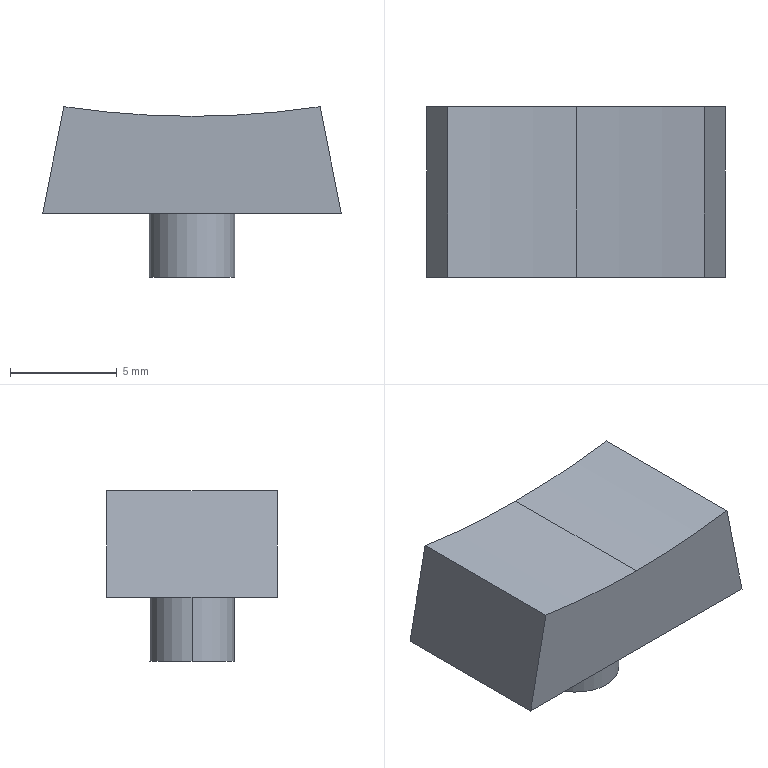Part | SolidWorks | features Extrusion 1, ICE 1 | 1 solid | 13 faces | box 14 x 8 x 8 mm | volume 507.497 mm3 | plane 7 | cylinder 6 | commonest cylinder face diameters 3 x2 4 x2 80 x2
STEP:
#1=CARTESIAN_POINT('',(-1.5,0.,-3.));
#2=VERTEX_POINT('',#1);
#3=CARTESIAN_POINT('',(1.5,0.,-3.));
#4=VERTEX_POINT('',#3);
#5=CARTESIAN_POINT('',(0.,0.,-3.));
#6=DIRECTION('',(0.,0.,1.));
#7=DIRECTION('',(1.,0.,0.));
#8=AXIS2_PLACEMENT_3D('',#5,#6,#7);
#9=CIRCLE('',#8,1.5);
#10=EDGE_CURVE('',#2,#4,#9,.T.);
#11=ORIENTED_EDGE('',*,*,#10,.F.);
#12=CARTESIAN_POINT('',(-1.5,0.,0.));
#13=VERTEX_POINT('',#12);
#14=CARTESIAN_POINT('',(-1.5,0.,-3.));
#15=DIRECTION('',(0.,0.,1.));
#16=VECTOR('',#15,1000.);
#17=LINE('',#14,#16);
#18=EDGE_CURVE('',#2,#13,#17,.T.);
#19=ORIENTED_EDGE('',*,*,#18,.T.);
#20=CARTESIAN_POINT('',(1.5,0.,0.));
#21=VERTEX_POINT('',#20);
#22=CARTESIAN_POINT('',(0.,0.,0.));
#23=DIRECTION('',(0.,0.,1.));
#24=DIRECTION('',(1.,0.,0.));
#25=AXIS2_PLACEMENT_3D('',#22,#23,#24);
#26=CIRCLE('',#25,1.5);
#27=EDGE_CURVE('',#13,#21,#26,.T.);
#28=ORIENTED_EDGE('',*,*,#27,.T.);
#29=CARTESIAN_POINT('',(1.5,0.,-3.));
#30=DIRECTION('',(0.,0.,1.));
#31=VECTOR('',#30,1000.);
#32=LINE('',#29,#31);
#33=EDGE_CURVE('',#4,#21,#32,.T.);
#34=ORIENTED_EDGE('',*,*,#33,.F.);
#35=EDGE_LOOP('',(#11,#19,#28,#34));
#36=FACE_OUTER_BOUND('',#35,.T.);
#37=CARTESIAN_POINT('',(0.,0.,-3.));
#38=DIRECTION('',(0.,0.,1.));
#39=DIRECTION('',(1.,0.,0.));
#40=AXIS2_PLACEMENT_3D('',#37,#38,#39);
#41=CYLINDRICAL_SURFACE('',#40,1.5);
#42=ADVANCED_FACE('',(#36),#41,.F.);
#43=CARTESIAN_POINT('',(2.,0.,-3.));
#44=VERTEX_POINT('',#43);
#45=CARTESIAN_POINT('',(-2.,0.,-3.));
#46=VERTEX_POINT('',#45);
#47=CARTESIAN_POINT('',(0.,0.,-3.));
#48=DIRECTION('',(0.,0.,1.));
#49=DIRECTION('',(1.,0.,0.));
#50=AXIS2_PLACEMENT_3D('',#47,#48,#49);
#51=CIRCLE('',#50,2.);
#52=EDGE_CURVE('',#44,#46,#51,.T.);
#53=ORIENTED_EDGE('',*,*,#52,.T.);
#54=CARTESIAN_POINT('',(-2.,0.,0.));
#55=VERTEX_POINT('',#54);
#56=CARTESIAN_POINT('',(-2.,0.,-3.));
#57=DIRECTION('',(0.,0.,1.));
#58=VECTOR('',#57,1000.);
#59=LINE('',#56,#58);
#60=EDGE_CURVE('',#46,#55,#59,.T.);
#61=ORIENTED_EDGE('',*,*,#60,.T.);
#62=CARTESIAN_POINT('',(2.,0.,0.));
#63=VERTEX_POINT('',#62);
#64=CARTESIAN_POINT('',(0.,0.,0.));
#65=DIRECTION('',(0.,0.,1.));
#66=DIRECTION('',(1.,0.,0.));
#67=AXIS2_PLACEMENT_3D('',#64,#65,#66);
#68=CIRCLE('',#67,2.);
#69=EDGE_CURVE('',#63,#55,#68,.T.);
#70=ORIENTED_EDGE('',*,*,#69,.F.);
#71=CARTESIAN_POINT('',(2.,0.,-3.));
#72=DIRECTION('',(0.,0.,1.));
#73=VECTOR('',#72,1000.);
#74=LINE('',#71,#73);
#75=EDGE_CURVE('',#44,#63,#74,.T.);
#76=ORIENTED_EDGE('',*,*,#75,.F.);
#77=EDGE_LOOP('',(#53,#61,#70,#76));
#78=FACE_OUTER_BOUND('',#77,.T.);
#79=CARTESIAN_POINT('',(0.,0.,-3.));
#80=DIRECTION('',(0.,0.,1.));
#81=DIRECTION('',(1.,0.,0.));
#82=AXIS2_PLACEMENT_3D('',#79,#80,#81);
#83=CYLINDRICAL_SURFACE('',#82,2.);
#84=ADVANCED_FACE('',(#78),#83,.T.);
#85=CARTESIAN_POINT('',(0.,4.,4.547));
#86=VERTEX_POINT('',#85);
#87=CARTESIAN_POINT('',(6.,4.,5.));
#88=VERTEX_POINT('',#87);
#89=CARTESIAN_POINT('',(0.,4.,44.547));
#90=DIRECTION('',(0.,-1.,0.));
#91=DIRECTION('',(0.,0.,-1.));
#92=AXIS2_PLACEMENT_3D('',#89,#90,#91);
#93=CIRCLE('',#92,40.);
#94=EDGE_CURVE('',#86,#88,#93,.T.);
#95=ORIENTED_EDGE('',*,*,#94,.F.);
#96=CARTESIAN_POINT('',(0.,-4.,4.547));
#97=VERTEX_POINT('',#96);
#98=CARTESIAN_POINT('',(0.,4.,4.547));
#99=DIRECTION('',(0.,-1.,0.));
#100=VECTOR('',#99,1000.);
#101=LINE('',#98,#100);
#102=EDGE_CURVE('',#86,#97,#101,.T.);
#103=ORIENTED_EDGE('',*,*,#102,.T.);
#104=CARTESIAN_POINT('',(6.,-4.,5.));
#105=VERTEX_POINT('',#104);
#106=CARTESIAN_POINT('',(0.,-4.,44.547));
#107=DIRECTION('',(0.,-1.,0.));
#108=DIRECTION('',(0.,0.,-1.));
#109=AXIS2_PLACEMENT_3D('',#106,#107,#108);
#110=CIRCLE('',#109,40.);
#111=EDGE_CURVE('',#97,#105,#110,.T.);
#112=ORIENTED_EDGE('',*,*,#111,.T.);
#113=CARTESIAN_POINT('',(6.,4.,5.));
#114=DIRECTION('',(0.,-1.,0.));
#115=VECTOR('',#114,1000.);
#116=LINE('',#113,#115);
#117=EDGE_CURVE('',#88,#105,#116,.T.);
#118=ORIENTED_EDGE('',*,*,#117,.F.);
#119=EDGE_LOOP('',(#95,#103,#112,#118));
#120=FACE_OUTER_BOUND('',#119,.T.);
#121=CARTESIAN_POINT('',(0.,4.,44.547));
#122=DIRECTION('',(0.,-1.,0.));
#123=DIRECTION('',(0.,0.,-1.));
#124=AXIS2_PLACEMENT_3D('',#121,#122,#123);
#125=CYLINDRICAL_SURFACE('',#124,40.);
#126=ADVANCED_FACE('',(#120),#125,.F.);
#127=CARTESIAN_POINT('',(7.,-4.,0.));
#128=VERTEX_POINT('',#127);
#129=CARTESIAN_POINT('',(7.,-4.,0.));
#130=DIRECTION('',(0.1961,0.,-0.9806));
#131=VECTOR('',#130,1000.);
#132=LINE('',#129,#131);
#133=EDGE_CURVE('',#105,#128,#132,.T.);
#134=ORIENTED_EDGE('',*,*,#133,.T.);
#135=CARTESIAN_POINT('',(7.,4.,0.));
#136=VERTEX_POINT('',#135);
#137=CARTESIAN_POINT('',(7.,4.,0.));
#138=DIRECTION('',(0.,-1.,0.));
#139=VECTOR('',#138,1000.);
#140=LINE('',#137,#139);
#141=EDGE_CURVE('',#136,#128,#140,.T.);
#142=ORIENTED_EDGE('',*,*,#141,.F.);
#143=CARTESIAN_POINT('',(7.,4.,0.));
#144=DIRECTION('',(0.1961,0.,-0.9806));
#145=VECTOR('',#144,1000.);
#146=LINE('',#143,#145);
#147=EDGE_CURVE('',#88,#136,#146,.T.);
#148=ORIENTED_EDGE('',*,*,#147,.F.);
#149=ORIENTED_EDGE('',*,*,#117,.T.);
#150=EDGE_LOOP('',(#134,#142,#148,#149));
#151=FACE_OUTER_BOUND('',#150,.T.);
#152=CARTESIAN_POINT('',(7.,4.,0.));
#153=DIRECTION('',(-0.9806,0.,-0.1961));
#154=DIRECTION('',(-0.1961,0.,0.9806));
#155=AXIS2_PLACEMENT_3D('',#152,#153,#154);
#156=PLANE('',#155);
#157=ADVANCED_FACE('',(#151),#156,.F.);
#158=ORIENTED_EDGE('',*,*,#69,.T.);
#159=CARTESIAN_POINT('',(0.,0.,0.));
#160=DIRECTION('',(0.,0.,1.));
#161=DIRECTION('',(1.,0.,0.));
#162=AXIS2_PLACEMENT_3D('',#159,#160,#161);
#163=CIRCLE('',#162,2.);
#164=EDGE_CURVE('',#55,#63,#163,.T.);
#165=ORIENTED_EDGE('',*,*,#164,.T.);
#166=EDGE_LOOP('',(#158,#165));
#167=FACE_BOUND('',#166,.T.);
#168=CARTESIAN_POINT('',(-7.,-4.,0.));
#169=VERTEX_POINT('',#168);
#170=CARTESIAN_POINT('',(7.,-4.,0.));
#171=DIRECTION('',(-1.,0.,0.));
#172=VECTOR('',#171,1000.);
#173=LINE('',#170,#172);
#174=EDGE_CURVE('',#128,#169,#173,.T.);
#175=ORIENTED_EDGE('',*,*,#174,.T.);
#176=CARTESIAN_POINT('',(-7.,4.,0.));
#177=VERTEX_POINT('',#176);
#178=CARTESIAN_POINT('',(-7.,4.,0.));
#179=DIRECTION('',(0.,-1.,0.));
#180=VECTOR('',#179,1000.);
#181=LINE('',#178,#180);
#182=EDGE_CURVE('',#177,#169,#181,.T.);
#183=ORIENTED_EDGE('',*,*,#182,.F.);
#184=CARTESIAN_POINT('',(7.,4.,0.));
#185=DIRECTION('',(-1.,0.,0.));
#186=VECTOR('',#185,1000.);
#187=LINE('',#184,#186);
#188=EDGE_CURVE('',#136,#177,#187,.T.);
#189=ORIENTED_EDGE('',*,*,#188,.F.);
#190=ORIENTED_EDGE('',*,*,#141,.T.);
#191=EDGE_LOOP('',(#175,#183,#189,#190));
#192=FACE_OUTER_BOUND('',#191,.T.);
#193=CARTESIAN_POINT('',(7.,4.,0.));
#194=DIRECTION('',(0.,0.,1.));
#195=DIRECTION('',(1.,0.,0.));
#196=AXIS2_PLACEMENT_3D('',#193,#194,#195);
#197=PLANE('',#196);
#198=ADVANCED_FACE('',(#167,#192),#197,.F.);
#199=CARTESIAN_POINT('',(-6.,-4.,5.));
#200=VERTEX_POINT('',#199);
#201=CARTESIAN_POINT('',(-7.,-4.,0.));
#202=DIRECTION('',(0.1961,0.,0.9806));
#203=VECTOR('',#202,1000.);
#204=LINE('',#201,#203);
#205=EDGE_CURVE('',#169,#200,#204,.T.);
#206=ORIENTED_EDGE('',*,*,#205,.T.);
#207=CARTESIAN_POINT('',(-6.,4.,5.));
#208=VERTEX_POINT('',#207);
#209=CARTESIAN_POINT('',(-6.,4.,5.));
#210=DIRECTION('',(0.,-1.,0.));
#211=VECTOR('',#210,1000.);
#212=LINE('',#209,#211);
#213=EDGE_CURVE('',#208,#200,#212,.T.);
#214=ORIENTED_EDGE('',*,*,#213,.F.);
#215=CARTESIAN_POINT('',(-7.,4.,0.));
#216=DIRECTION('',(0.1961,0.,0.9806));
#217=VECTOR('',#216,1000.);
#218=LINE('',#215,#217);
#219=EDGE_CURVE('',#177,#208,#218,.T.);
#220=ORIENTED_EDGE('',*,*,#219,.F.);
#221=ORIENTED_EDGE('',*,*,#182,.T.);
#222=EDGE_LOOP('',(#206,#214,#220,#221));
#223=FACE_OUTER_BOUND('',#222,.T.);
#224=CARTESIAN_POINT('',(-7.,4.,0.));
#225=DIRECTION('',(0.9806,0.,-0.1961));
#226=DIRECTION('',(-0.1961,0.,-0.9806));
#227=AXIS2_PLACEMENT_3D('',#224,#225,#226);
#228=PLANE('',#227);
#229=ADVANCED_FACE('',(#223),#228,.F.);
#230=ORIENTED_EDGE('',*,*,#102,.F.);
#231=CARTESIAN_POINT('',(0.,4.,44.547));
#232=DIRECTION('',(0.,-1.,0.));
#233=DIRECTION('',(0.,0.,-1.));
#234=AXIS2_PLACEMENT_3D('',#231,#232,#233);
#235=CIRCLE('',#234,40.);
#236=EDGE_CURVE('',#208,#86,#235,.T.);
#237=ORIENTED_EDGE('',*,*,#236,.F.);
#238=ORIENTED_EDGE('',*,*,#213,.T.);
#239=CARTESIAN_POINT('',(0.,-4.,44.547));
#240=DIRECTION('',(0.,-1.,0.));
#241=DIRECTION('',(0.,0.,-1.));
#242=AXIS2_PLACEMENT_3D('',#239,#240,#241);
#243=CIRCLE('',#242,40.);
#244=EDGE_CURVE('',#200,#97,#243,.T.);
#245=ORIENTED_EDGE('',*,*,#244,.T.);
#246=EDGE_LOOP('',(#230,#237,#238,#245));
#247=FACE_OUTER_BOUND('',#246,.T.);
#248=CARTESIAN_POINT('',(0.,4.,44.547));
#249=DIRECTION('',(0.,-1.,0.));
#250=DIRECTION('',(0.,0.,-1.));
#251=AXIS2_PLACEMENT_3D('',#248,#249,#250);
#252=CYLINDRICAL_SURFACE('',#251,40.);
#253=ADVANCED_FACE('',(#247),#252,.F.);
#254=ORIENTED_EDGE('',*,*,#147,.T.);
#255=ORIENTED_EDGE('',*,*,#188,.T.);
#256=ORIENTED_EDGE('',*,*,#219,.T.);
#257=ORIENTED_EDGE('',*,*,#236,.T.);
#258=ORIENTED_EDGE('',*,*,#94,.T.);
#259=EDGE_LOOP('',(#254,#255,#256,#257,#258));
#260=FACE_OUTER_BOUND('',#259,.T.);
#261=CARTESIAN_POINT('',(0.,4.,44.547));
#262=DIRECTION('',(0.,-1.,0.));
#263=DIRECTION('',(0.,0.,-1.));
#264=AXIS2_PLACEMENT_3D('',#261,#262,#263);
#265=PLANE('',#264);
#266=ADVANCED_FACE('',(#260),#265,.F.);
#267=ORIENTED_EDGE('',*,*,#133,.F.);
#268=ORIENTED_EDGE('',*,*,#111,.F.);
#269=ORIENTED_EDGE('',*,*,#244,.F.);
#270=ORIENTED_EDGE('',*,*,#205,.F.);
#271=ORIENTED_EDGE('',*,*,#174,.F.);
#272=EDGE_LOOP('',(#267,#268,#269,#270,#271));
#273=FACE_OUTER_BOUND('',#272,.T.);
#274=CARTESIAN_POINT('',(0.,-4.,44.547));
#275=DIRECTION('',(0.,-1.,0.));
#276=DIRECTION('',(0.,0.,-1.));
#277=AXIS2_PLACEMENT_3D('',#274,#275,#276);
#278=PLANE('',#277);
#279=ADVANCED_FACE('',(#273),#278,.T.);
#280=ORIENTED_EDGE('',*,*,#60,.F.);
#281=CARTESIAN_POINT('',(0.,0.,-3.));
#282=DIRECTION('',(0.,0.,1.));
#283=DIRECTION('',(1.,0.,0.));
#284=AXIS2_PLACEMENT_3D('',#281,#282,#283);
#285=CIRCLE('',#284,2.);
#286=EDGE_CURVE('',#46,#44,#285,.T.);
#287=ORIENTED_EDGE('',*,*,#286,.T.);
#288=ORIENTED_EDGE('',*,*,#75,.T.);
#289=ORIENTED_EDGE('',*,*,#164,.F.);
#290=EDGE_LOOP('',(#280,#287,#288,#289));
#291=FACE_OUTER_BOUND('',#290,.T.);
#292=CARTESIAN_POINT('',(0.,0.,-3.));
#293=DIRECTION('',(0.,0.,1.));
#294=DIRECTION('',(1.,0.,0.));
#295=AXIS2_PLACEMENT_3D('',#292,#293,#294);
#296=CYLINDRICAL_SURFACE('',#295,2.);
#297=ADVANCED_FACE('',(#291),#296,.T.);
#298=CARTESIAN_POINT('',(0.,0.,-3.));
#299=DIRECTION('',(0.,0.,1.));
#300=DIRECTION('',(1.,0.,0.));
#301=AXIS2_PLACEMENT_3D('',#298,#299,#300);
#302=CIRCLE('',#301,1.5);
#303=EDGE_CURVE('',#4,#2,#302,.T.);
#304=ORIENTED_EDGE('',*,*,#303,.T.);
#305=ORIENTED_EDGE('',*,*,#10,.T.);
#306=EDGE_LOOP('',(#304,#305));
#307=FACE_BOUND('',#306,.T.);
#308=ORIENTED_EDGE('',*,*,#52,.F.);
#309=ORIENTED_EDGE('',*,*,#286,.F.);
#310=EDGE_LOOP('',(#308,#309));
#311=FACE_OUTER_BOUND('',#310,.T.);
#312=CARTESIAN_POINT('',(0.,0.,-3.));
#313=DIRECTION('',(0.,0.,1.));
#314=DIRECTION('',(1.,0.,0.));
#315=AXIS2_PLACEMENT_3D('',#312,#313,#314);
#316=PLANE('',#315);
#317=ADVANCED_FACE('',(#307,#311),#316,.F.);
#318=ORIENTED_EDGE('',*,*,#18,.F.);
#319=ORIENTED_EDGE('',*,*,#303,.F.);
#320=ORIENTED_EDGE('',*,*,#33,.T.);
#321=CARTESIAN_POINT('',(0.,0.,0.));
#322=DIRECTION('',(0.,0.,1.));
#323=DIRECTION('',(1.,0.,0.));
#324=AXIS2_PLACEMENT_3D('',#321,#322,#323);
#325=CIRCLE('',#324,1.5);
#326=EDGE_CURVE('',#21,#13,#325,.T.);
#327=ORIENTED_EDGE('',*,*,#326,.T.);
#328=EDGE_LOOP('',(#318,#319,#320,#327));
#329=FACE_OUTER_BOUND('',#328,.T.);
#330=CARTESIAN_POINT('',(0.,0.,-3.));
#331=DIRECTION('',(0.,0.,1.));
#332=DIRECTION('',(1.,0.,0.));
#333=AXIS2_PLACEMENT_3D('',#330,#331,#332);
#334=CYLINDRICAL_SURFACE('',#333,1.5);
#335=ADVANCED_FACE('',(#329),#334,.F.);
#336=ORIENTED_EDGE('',*,*,#326,.F.);
#337=ORIENTED_EDGE('',*,*,#27,.F.);
#338=EDGE_LOOP('',(#336,#337));
#339=FACE_OUTER_BOUND('',#338,.T.);
#340=CARTESIAN_POINT('',(7.,4.,0.));
#341=DIRECTION('',(0.,0.,1.));
#342=DIRECTION('',(1.,0.,0.));
#343=AXIS2_PLACEMENT_3D('',#340,#341,#342);
#344=PLANE('',#343);
#345=ADVANCED_FACE('',(#339),#344,.F.);
#346=CLOSED_SHELL('',(#42,#84,#126,#157,#198,#229,#253,#266,#279,#297,#317,#335,#345));
#347=MANIFOLD_SOLID_BREP('',#346);
#348=CARTESIAN_POINT('',(0.,0.,0.));
#349=DIRECTION('',(0.,0.,1.));
#350=DIRECTION('',(1.,0.,0.));
#351=AXIS2_PLACEMENT_3D('',#348,#349,#350);
#352=(LENGTH_UNIT()NAMED_UNIT(*)SI_UNIT(.MILLI.,.METRE.));
#353=UNCERTAINTY_MEASURE_WITH_UNIT(LENGTH_MEASURE(0.00001),#352,'','');
#354=(NAMED_UNIT(*)PLANE_ANGLE_UNIT()SI_UNIT($,.RADIAN.));
#355=(NAMED_UNIT(*)SI_UNIT($,.STERADIAN.)SOLID_ANGLE_UNIT());
#356=(GEOMETRIC_REPRESENTATION_CONTEXT(3)GLOBAL_UNCERTAINTY_ASSIGNED_CONTEXT((#353))GLOBAL_UNIT_ASSIGNED_CONTEXT((#352,#354,#355))REPRESENTATION_CONTEXT('',''));
#357=ADVANCED_BREP_SHAPE_REPRESENTATION('',(#347,#351),#356);